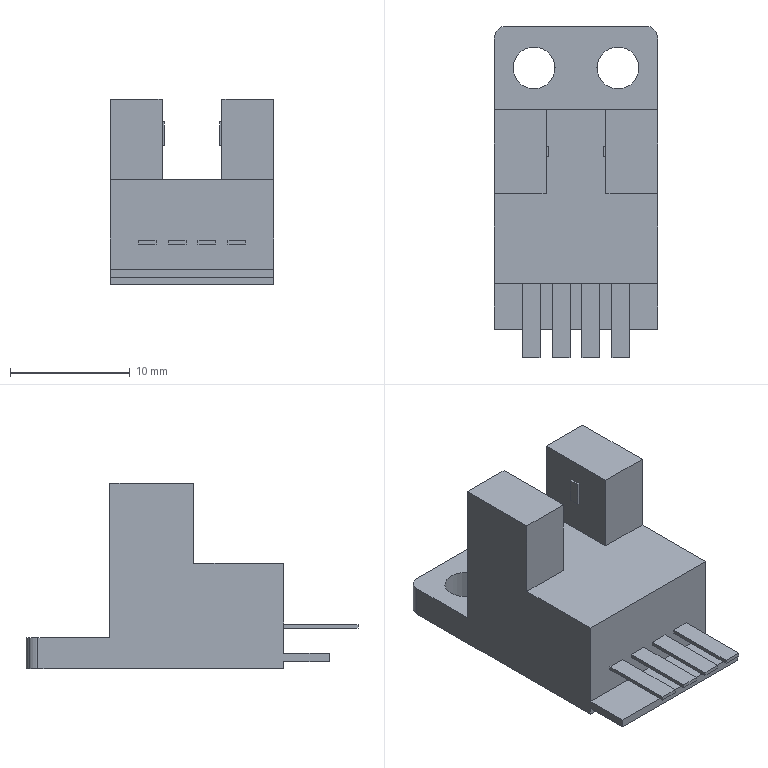Part | NX | 1 solid | 56 faces | box 13.6 x 27.7 x 15.5 mm | volume 2383 mm3 | plane 48 | cylinder 8 | commonest cylinder face diameters 2 x4 3.5 x4